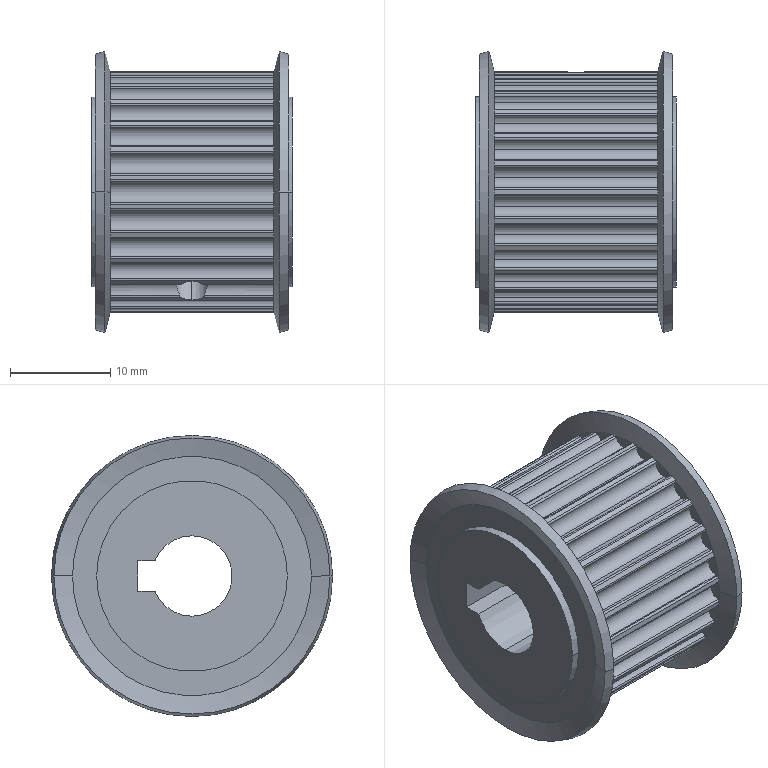Part | NX | features BREP 3 | 3 solids | 264 faces | box 20 x 28 x 28 mm | volume 7174 mm3 | cylinder 150 | plane 90 | cone 24 | commonest cylinder face diameters 0.34 x69 2.06 x40 24.07 x26 3.242 x4 4 x4 19 x4